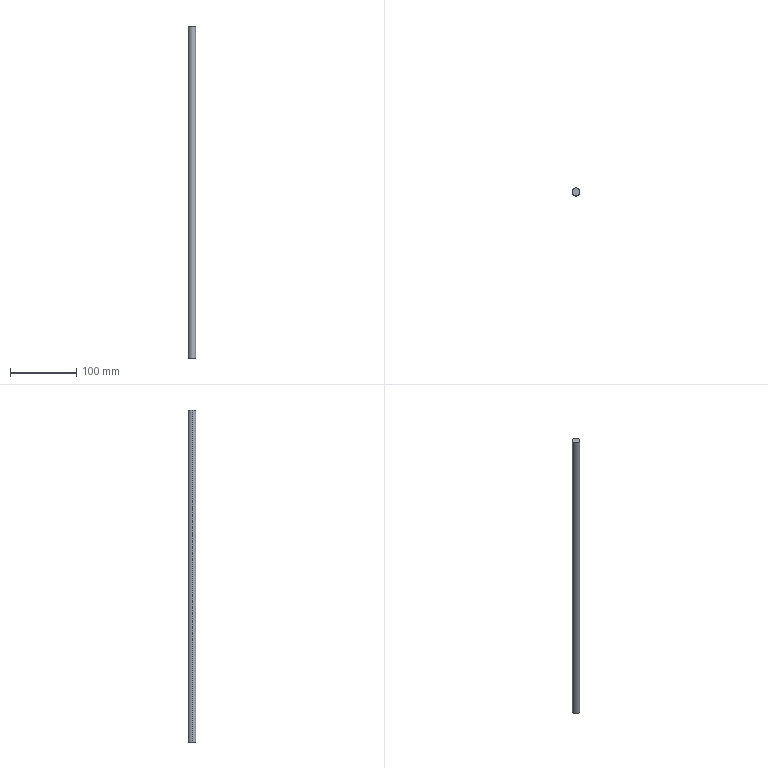Part | STEP file | CF881.03.25 | 1 solid | 4 faces | box 11.5 x 11.5 x 500 mm | volume 51934 mm3 | cylinder 2 | plane 2 | commonest cylinder face diameters 11.5 x2
STEP:
#1=CARTESIAN_POINT('',(5.75,0.,500.));
#2=VERTEX_POINT('',#1);
#3=CARTESIAN_POINT('',(-5.75,0.,500.));
#4=VERTEX_POINT('',#3);
#5=CARTESIAN_POINT('',(0.,0.,500.));
#6=DIRECTION('',(0.,0.,1.));
#7=DIRECTION('',(1.,0.,0.));
#8=AXIS2_PLACEMENT_3D('',#5,#6,#7);
#9=CIRCLE('',#8,5.75);
#10=EDGE_CURVE('',#2,#4,#9,.T.);
#11=ORIENTED_EDGE('',*,*,#10,.F.);
#12=CARTESIAN_POINT('',(5.75,0.,0.));
#13=VERTEX_POINT('',#12);
#14=CARTESIAN_POINT('',(5.75,0.,500.));
#15=DIRECTION('',(0.,0.,-1.));
#16=VECTOR('',#15,1000.);
#17=LINE('',#14,#16);
#18=EDGE_CURVE('',#2,#13,#17,.T.);
#19=ORIENTED_EDGE('',*,*,#18,.T.);
#20=CARTESIAN_POINT('',(-5.75,0.,0.));
#21=VERTEX_POINT('',#20);
#22=CARTESIAN_POINT('',(0.,0.,0.));
#23=DIRECTION('',(0.,0.,1.));
#24=DIRECTION('',(1.,0.,0.));
#25=AXIS2_PLACEMENT_3D('',#22,#23,#24);
#26=CIRCLE('',#25,5.75);
#27=EDGE_CURVE('',#13,#21,#26,.T.);
#28=ORIENTED_EDGE('',*,*,#27,.T.);
#29=CARTESIAN_POINT('',(-5.75,0.,500.));
#30=DIRECTION('',(0.,0.,-1.));
#31=VECTOR('',#30,1000.);
#32=LINE('',#29,#31);
#33=EDGE_CURVE('',#4,#21,#32,.T.);
#34=ORIENTED_EDGE('',*,*,#33,.F.);
#35=EDGE_LOOP('',(#11,#19,#28,#34));
#36=FACE_OUTER_BOUND('',#35,.T.);
#37=CARTESIAN_POINT('',(0.,0.,500.));
#38=DIRECTION('',(0.,0.,-1.));
#39=DIRECTION('',(-1.,0.,0.));
#40=AXIS2_PLACEMENT_3D('',#37,#38,#39);
#41=CYLINDRICAL_SURFACE('',#40,5.75);
#42=ADVANCED_FACE('',(#36),#41,.T.);
#43=ORIENTED_EDGE('',*,*,#18,.F.);
#44=CARTESIAN_POINT('',(0.,0.,500.));
#45=DIRECTION('',(0.,0.,1.));
#46=DIRECTION('',(1.,0.,0.));
#47=AXIS2_PLACEMENT_3D('',#44,#45,#46);
#48=CIRCLE('',#47,5.75);
#49=EDGE_CURVE('',#4,#2,#48,.T.);
#50=ORIENTED_EDGE('',*,*,#49,.F.);
#51=ORIENTED_EDGE('',*,*,#33,.T.);
#52=CARTESIAN_POINT('',(0.,0.,0.));
#53=DIRECTION('',(0.,0.,1.));
#54=DIRECTION('',(1.,0.,0.));
#55=AXIS2_PLACEMENT_3D('',#52,#53,#54);
#56=CIRCLE('',#55,5.75);
#57=EDGE_CURVE('',#21,#13,#56,.T.);
#58=ORIENTED_EDGE('',*,*,#57,.T.);
#59=EDGE_LOOP('',(#43,#50,#51,#58));
#60=FACE_OUTER_BOUND('',#59,.T.);
#61=CARTESIAN_POINT('',(0.,0.,500.));
#62=DIRECTION('',(0.,0.,-1.));
#63=DIRECTION('',(-1.,0.,0.));
#64=AXIS2_PLACEMENT_3D('',#61,#62,#63);
#65=CYLINDRICAL_SURFACE('',#64,5.75);
#66=ADVANCED_FACE('',(#60),#65,.T.);
#67=ORIENTED_EDGE('',*,*,#49,.T.);
#68=ORIENTED_EDGE('',*,*,#10,.T.);
#69=EDGE_LOOP('',(#67,#68));
#70=FACE_OUTER_BOUND('',#69,.T.);
#71=CARTESIAN_POINT('',(0.,0.,500.));
#72=DIRECTION('',(0.,0.,1.));
#73=DIRECTION('',(1.,0.,0.));
#74=AXIS2_PLACEMENT_3D('',#71,#72,#73);
#75=PLANE('',#74);
#76=ADVANCED_FACE('',(#70),#75,.T.);
#77=ORIENTED_EDGE('',*,*,#57,.F.);
#78=ORIENTED_EDGE('',*,*,#27,.F.);
#79=EDGE_LOOP('',(#77,#78));
#80=FACE_OUTER_BOUND('',#79,.T.);
#81=CARTESIAN_POINT('',(0.,0.,0.));
#82=DIRECTION('',(0.,0.,1.));
#83=DIRECTION('',(1.,0.,0.));
#84=AXIS2_PLACEMENT_3D('',#81,#82,#83);
#85=PLANE('',#84);
#86=ADVANCED_FACE('',(#80),#85,.F.);
#87=CLOSED_SHELL('',(#42,#66,#76,#86));
#88=MANIFOLD_SOLID_BREP('',#87);
#89=CARTESIAN_POINT('',(0.,0.,0.));
#90=DIRECTION('',(0.,0.,1.));
#91=DIRECTION('',(1.,0.,0.));
#92=AXIS2_PLACEMENT_3D('',#89,#90,#91);
#93=(LENGTH_UNIT()NAMED_UNIT(*)SI_UNIT(.MILLI.,.METRE.));
#94=UNCERTAINTY_MEASURE_WITH_UNIT(LENGTH_MEASURE(0.00001),#93,'','');
#95=(NAMED_UNIT(*)PLANE_ANGLE_UNIT()SI_UNIT($,.RADIAN.));
#96=(NAMED_UNIT(*)SI_UNIT($,.STERADIAN.)SOLID_ANGLE_UNIT());
#97=(GEOMETRIC_REPRESENTATION_CONTEXT(3)GLOBAL_UNCERTAINTY_ASSIGNED_CONTEXT((#94))GLOBAL_UNIT_ASSIGNED_CONTEXT((#93,#95,#96))REPRESENTATION_CONTEXT('',''));
#98=ADVANCED_BREP_SHAPE_REPRESENTATION('',(#88,#92),#97);